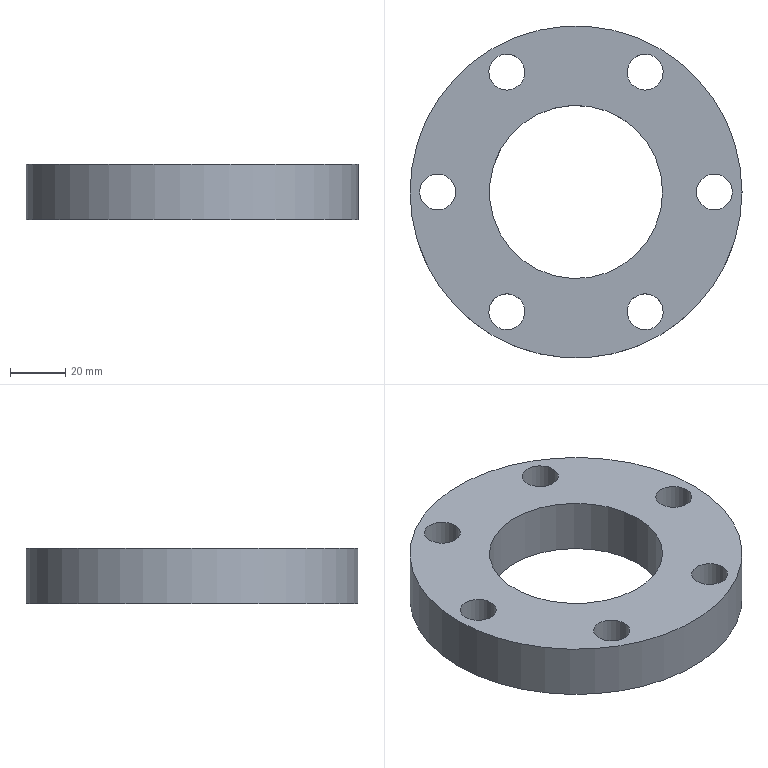CAM job | NX | 3-axis milling, drilling | part box 120 x 120 x 20 mm | stock box 120 x 120 x 20 mm
Tools:
number,name,description,diameter,corner_radius,flute_length,length,flutes
1,ZXZ,Milling Tool-5 Parameters,6.0,0.0,50.0,75.0,2
7,D6A45,Milling Tool-5 Parameters,6.0,0.0,3.0,3.0,2
3,13.0ZT,Drilling Tool,13.0,0.0,35.0,50.0,2
Operations:
program,operation,operation_type,tool,method,geometry_group,spindle_rpm,surface_speed,feed_per_tooth,feed_cut,feed_plunge,cut_length_mm,path_length_mm,cut_time_min,machine_time_min
1,DRILLING,Operation,ZXZ,METHOD,A,3000.0,56.0,0.0333,200.0,0.0,24.0,453.45,0.12,0.1629
1,DRILLING_COPY,Operation,13.0ZT,METHOD,A,800.0,32.0,0.0938,150.0,0.0,170.434,746.317,1.136,1.194
1,ZLEVEL_PROFILE_1_COPY_1,ZLevelMilling,D6A45,METHOD,A,7500.0,141.0,0.0667,1000.0,100.0,246.048,1479.531,0.246,0.3694